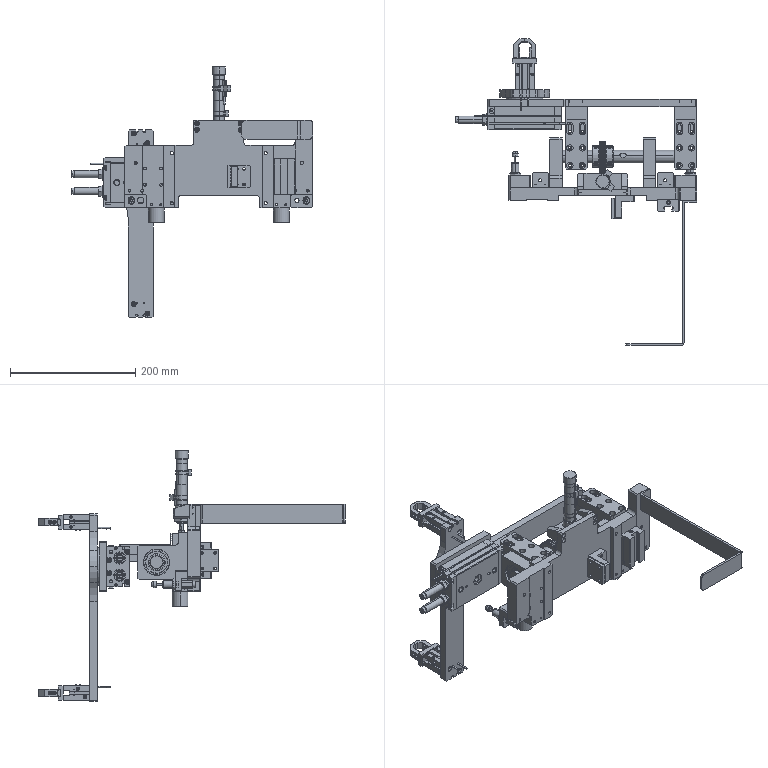Part | SolidWorks | features InContextFeatHolder 12, ReferencePattern 4, CompositeCurve 2, MirrorCompFeat 1 | 92 solids | 3667 faces | volume 1868083 mm3 | plane 1528 | cylinder 1473 | cone 466 | sphere 120 | torus 80 | commonest cylinder face diameters 0.5 x124 10 x85 4.2 x74 5.5 x56 29.9 x54 32.1 x54